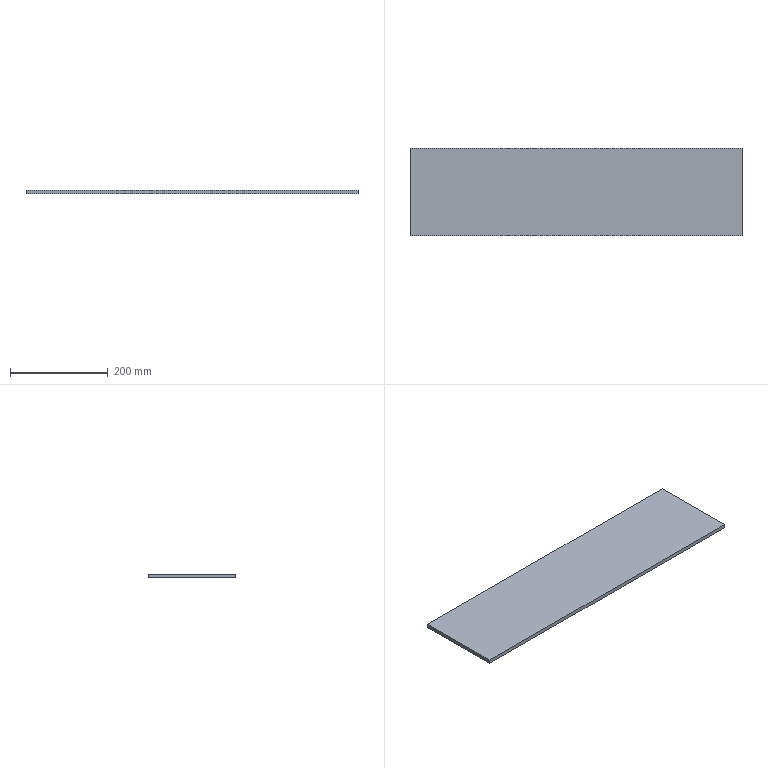Part | STEP file | 04-Steel plate 680x180x8 | 1 solid | 6 faces | box 680 x 180 x 8 mm | volume 979200 mm3 | plane 6
STEP:
#1=CARTESIAN_POINT('',(0.,0.,0.));
#2=DIRECTION('',(0.,0.,1.));
#3=DIRECTION('',(1.,0.,0.));
#4=AXIS2_PLACEMENT_3D('',#1,#2,#3);
#5=CARTESIAN_POINT('',(0.,0.,0.));
#6=VERTEX_POINT('',#5);
#7=CARTESIAN_POINT('',(0.,-180.,0.));
#8=VERTEX_POINT('',#7);
#9=CARTESIAN_POINT('',(0.,0.,0.));
#10=DIRECTION('',(0.,-1.,0.));
#11=VECTOR('',#10,1.);
#12=LINE('',#9,#11);
#13=CARTESIAN_POINT('',(0.,0.,8.));
#14=DIRECTION('',(1.,0.,0.));
#15=DIRECTION('',(0.,1.,0.));
#16=AXIS2_PLACEMENT_3D('',#13,#14,#15);
#17=PLANE('',#16);
#18=CARTESIAN_POINT('',(0.,-8.));
#19=DIRECTION('',(-1.,0.));
#20=VECTOR('',#19,1.);
#21=LINE('',#18,#20);
#22=(GEOMETRIC_REPRESENTATION_CONTEXT(2)PARAMETRIC_REPRESENTATION_CONTEXT()REPRESENTATION_CONTEXT('',''));
#23=DEFINITIONAL_REPRESENTATION('',(#21),#22);
#24=PCURVE('',#17,#23);
#25=CARTESIAN_POINT('',(0.,0.,0.));
#26=DIRECTION('',(0.,0.,1.));
#27=DIRECTION('',(1.,0.,0.));
#28=AXIS2_PLACEMENT_3D('',#25,#26,#27);
#29=PLANE('',#28);
#30=CARTESIAN_POINT('',(0.,0.));
#31=DIRECTION('',(0.,-1.));
#32=VECTOR('',#31,1.);
#33=LINE('',#30,#32);
#34=(GEOMETRIC_REPRESENTATION_CONTEXT(2)PARAMETRIC_REPRESENTATION_CONTEXT()REPRESENTATION_CONTEXT('',''));
#35=DEFINITIONAL_REPRESENTATION('',(#33),#34);
#36=PCURVE('',#29,#35);
#37=SURFACE_CURVE('',#12,(#24,#36),.PCURVE_S1.);
#38=EDGE_CURVE('',#6,#8,#37,.T.);
#39=ORIENTED_EDGE('',*,*,#38,.T.);
#40=CARTESIAN_POINT('',(0.,-180.,8.));
#41=VERTEX_POINT('',#40);
#42=CARTESIAN_POINT('',(0.,-180.,8.));
#43=DIRECTION('',(0.,0.,-1.));
#44=VECTOR('',#43,1.);
#45=LINE('',#42,#44);
#46=CARTESIAN_POINT('',(-180.,0.));
#47=DIRECTION('',(0.,-1.));
#48=VECTOR('',#47,1.);
#49=LINE('',#46,#48);
#50=(GEOMETRIC_REPRESENTATION_CONTEXT(2)PARAMETRIC_REPRESENTATION_CONTEXT()REPRESENTATION_CONTEXT('',''));
#51=DEFINITIONAL_REPRESENTATION('',(#49),#50);
#52=PCURVE('',#17,#51);
#53=CARTESIAN_POINT('',(0.,-180.,8.));
#54=DIRECTION('',(0.,1.,0.));
#55=DIRECTION('',(0.,0.,1.));
#56=AXIS2_PLACEMENT_3D('',#53,#54,#55);
#57=PLANE('',#56);
#58=CARTESIAN_POINT('',(0.,0.));
#59=DIRECTION('',(-1.,0.));
#60=VECTOR('',#59,1.);
#61=LINE('',#58,#60);
#62=(GEOMETRIC_REPRESENTATION_CONTEXT(2)PARAMETRIC_REPRESENTATION_CONTEXT()REPRESENTATION_CONTEXT('',''));
#63=DEFINITIONAL_REPRESENTATION('',(#61),#62);
#64=PCURVE('',#57,#63);
#65=SURFACE_CURVE('',#45,(#52,#64),.PCURVE_S1.);
#66=EDGE_CURVE('',#41,#8,#65,.T.);
#67=ORIENTED_EDGE('',*,*,#66,.F.);
#68=CARTESIAN_POINT('',(0.,0.,8.));
#69=VERTEX_POINT('',#68);
#70=CARTESIAN_POINT('',(0.,0.,8.));
#71=DIRECTION('',(0.,-1.,0.));
#72=VECTOR('',#71,1.);
#73=LINE('',#70,#72);
#74=CARTESIAN_POINT('',(0.,0.));
#75=DIRECTION('',(-1.,0.));
#76=VECTOR('',#75,1.);
#77=LINE('',#74,#76);
#78=(GEOMETRIC_REPRESENTATION_CONTEXT(2)PARAMETRIC_REPRESENTATION_CONTEXT()REPRESENTATION_CONTEXT('',''));
#79=DEFINITIONAL_REPRESENTATION('',(#77),#78);
#80=PCURVE('',#17,#79);
#81=CARTESIAN_POINT('',(0.,0.,8.));
#82=DIRECTION('',(0.,0.,1.));
#83=DIRECTION('',(1.,0.,0.));
#84=AXIS2_PLACEMENT_3D('',#81,#82,#83);
#85=PLANE('',#84);
#86=CARTESIAN_POINT('',(0.,0.));
#87=DIRECTION('',(0.,-1.));
#88=VECTOR('',#87,1.);
#89=LINE('',#86,#88);
#90=(GEOMETRIC_REPRESENTATION_CONTEXT(2)PARAMETRIC_REPRESENTATION_CONTEXT()REPRESENTATION_CONTEXT('',''));
#91=DEFINITIONAL_REPRESENTATION('',(#89),#90);
#92=PCURVE('',#85,#91);
#93=SURFACE_CURVE('',#73,(#80,#92),.PCURVE_S1.);
#94=EDGE_CURVE('',#69,#41,#93,.T.);
#95=ORIENTED_EDGE('',*,*,#94,.F.);
#96=CARTESIAN_POINT('',(0.,0.,8.));
#97=DIRECTION('',(0.,0.,-1.));
#98=VECTOR('',#97,1.);
#99=LINE('',#96,#98);
#100=CARTESIAN_POINT('',(0.,0.));
#101=DIRECTION('',(0.,-1.));
#102=VECTOR('',#101,1.);
#103=LINE('',#100,#102);
#104=(GEOMETRIC_REPRESENTATION_CONTEXT(2)PARAMETRIC_REPRESENTATION_CONTEXT()REPRESENTATION_CONTEXT('',''));
#105=DEFINITIONAL_REPRESENTATION('',(#103),#104);
#106=PCURVE('',#17,#105);
#107=CARTESIAN_POINT('',(0.,0.,8.));
#108=DIRECTION('',(0.,-1.,0.));
#109=DIRECTION('',(0.,0.,-1.));
#110=AXIS2_PLACEMENT_3D('',#107,#108,#109);
#111=PLANE('',#110);
#112=CARTESIAN_POINT('',(0.,0.));
#113=DIRECTION('',(1.,0.));
#114=VECTOR('',#113,1.);
#115=LINE('',#112,#114);
#116=(GEOMETRIC_REPRESENTATION_CONTEXT(2)PARAMETRIC_REPRESENTATION_CONTEXT()REPRESENTATION_CONTEXT('',''));
#117=DEFINITIONAL_REPRESENTATION('',(#115),#116);
#118=PCURVE('',#111,#117);
#119=SURFACE_CURVE('',#99,(#106,#118),.PCURVE_S1.);
#120=EDGE_CURVE('',#69,#6,#119,.T.);
#121=ORIENTED_EDGE('',*,*,#120,.T.);
#122=EDGE_LOOP('',(#39,#67,#95,#121));
#123=FACE_BOUND('',#122,.T.);
#124=ADVANCED_FACE('',(#123),#17,.F.);
#125=CARTESIAN_POINT('',(680.,-180.,0.));
#126=VERTEX_POINT('',#125);
#127=CARTESIAN_POINT('',(0.,-180.,0.));
#128=DIRECTION('',(1.,0.,0.));
#129=VECTOR('',#128,1.);
#130=LINE('',#127,#129);
#131=CARTESIAN_POINT('',(-8.,0.));
#132=DIRECTION('',(0.,1.));
#133=VECTOR('',#132,1.);
#134=LINE('',#131,#133);
#135=(GEOMETRIC_REPRESENTATION_CONTEXT(2)PARAMETRIC_REPRESENTATION_CONTEXT()REPRESENTATION_CONTEXT('',''));
#136=DEFINITIONAL_REPRESENTATION('',(#134),#135);
#137=PCURVE('',#57,#136);
#138=CARTESIAN_POINT('',(0.,-180.));
#139=DIRECTION('',(1.,0.));
#140=VECTOR('',#139,1.);
#141=LINE('',#138,#140);
#142=(GEOMETRIC_REPRESENTATION_CONTEXT(2)PARAMETRIC_REPRESENTATION_CONTEXT()REPRESENTATION_CONTEXT('',''));
#143=DEFINITIONAL_REPRESENTATION('',(#141),#142);
#144=PCURVE('',#29,#143);
#145=SURFACE_CURVE('',#130,(#137,#144),.PCURVE_S1.);
#146=EDGE_CURVE('',#8,#126,#145,.T.);
#147=ORIENTED_EDGE('',*,*,#146,.T.);
#148=CARTESIAN_POINT('',(680.,-180.,8.));
#149=VERTEX_POINT('',#148);
#150=CARTESIAN_POINT('',(680.,-180.,8.));
#151=DIRECTION('',(0.,0.,-1.));
#152=VECTOR('',#151,1.);
#153=LINE('',#150,#152);
#154=CARTESIAN_POINT('',(0.,680.));
#155=DIRECTION('',(-1.,0.));
#156=VECTOR('',#155,1.);
#157=LINE('',#154,#156);
#158=(GEOMETRIC_REPRESENTATION_CONTEXT(2)PARAMETRIC_REPRESENTATION_CONTEXT()REPRESENTATION_CONTEXT('',''));
#159=DEFINITIONAL_REPRESENTATION('',(#157),#158);
#160=PCURVE('',#57,#159);
#161=CARTESIAN_POINT('',(680.,0.,8.));
#162=DIRECTION('',(-1.,0.,0.));
#163=DIRECTION('',(0.,0.,1.));
#164=AXIS2_PLACEMENT_3D('',#161,#162,#163);
#165=PLANE('',#164);
#166=CARTESIAN_POINT('',(0.,-180.));
#167=DIRECTION('',(-1.,0.));
#168=VECTOR('',#167,1.);
#169=LINE('',#166,#168);
#170=(GEOMETRIC_REPRESENTATION_CONTEXT(2)PARAMETRIC_REPRESENTATION_CONTEXT()REPRESENTATION_CONTEXT('',''));
#171=DEFINITIONAL_REPRESENTATION('',(#169),#170);
#172=PCURVE('',#165,#171);
#173=SURFACE_CURVE('',#153,(#160,#172),.PCURVE_S1.);
#174=EDGE_CURVE('',#149,#126,#173,.T.);
#175=ORIENTED_EDGE('',*,*,#174,.F.);
#176=CARTESIAN_POINT('',(0.,-180.,8.));
#177=DIRECTION('',(1.,0.,0.));
#178=VECTOR('',#177,1.);
#179=LINE('',#176,#178);
#180=CARTESIAN_POINT('',(0.,0.));
#181=DIRECTION('',(0.,1.));
#182=VECTOR('',#181,1.);
#183=LINE('',#180,#182);
#184=(GEOMETRIC_REPRESENTATION_CONTEXT(2)PARAMETRIC_REPRESENTATION_CONTEXT()REPRESENTATION_CONTEXT('',''));
#185=DEFINITIONAL_REPRESENTATION('',(#183),#184);
#186=PCURVE('',#57,#185);
#187=CARTESIAN_POINT('',(0.,-180.));
#188=DIRECTION('',(1.,0.));
#189=VECTOR('',#188,1.);
#190=LINE('',#187,#189);
#191=(GEOMETRIC_REPRESENTATION_CONTEXT(2)PARAMETRIC_REPRESENTATION_CONTEXT()REPRESENTATION_CONTEXT('',''));
#192=DEFINITIONAL_REPRESENTATION('',(#190),#191);
#193=PCURVE('',#85,#192);
#194=SURFACE_CURVE('',#179,(#186,#193),.PCURVE_S1.);
#195=EDGE_CURVE('',#41,#149,#194,.T.);
#196=ORIENTED_EDGE('',*,*,#195,.F.);
#197=ORIENTED_EDGE('',*,*,#66,.T.);
#198=EDGE_LOOP('',(#147,#175,#196,#197));
#199=FACE_BOUND('',#198,.T.);
#200=ADVANCED_FACE('',(#199),#57,.F.);
#201=CARTESIAN_POINT('',(680.,0.,0.));
#202=VERTEX_POINT('',#201);
#203=CARTESIAN_POINT('',(680.,0.,0.));
#204=DIRECTION('',(0.,1.,0.));
#205=VECTOR('',#204,1.);
#206=LINE('',#203,#205);
#207=CARTESIAN_POINT('',(-8.,0.));
#208=DIRECTION('',(0.,1.));
#209=VECTOR('',#208,1.);
#210=LINE('',#207,#209);
#211=(GEOMETRIC_REPRESENTATION_CONTEXT(2)PARAMETRIC_REPRESENTATION_CONTEXT()REPRESENTATION_CONTEXT('',''));
#212=DEFINITIONAL_REPRESENTATION('',(#210),#211);
#213=PCURVE('',#165,#212);
#214=CARTESIAN_POINT('',(680.,0.));
#215=DIRECTION('',(0.,1.));
#216=VECTOR('',#215,1.);
#217=LINE('',#214,#216);
#218=(GEOMETRIC_REPRESENTATION_CONTEXT(2)PARAMETRIC_REPRESENTATION_CONTEXT()REPRESENTATION_CONTEXT('',''));
#219=DEFINITIONAL_REPRESENTATION('',(#217),#218);
#220=PCURVE('',#29,#219);
#221=SURFACE_CURVE('',#206,(#213,#220),.PCURVE_S1.);
#222=EDGE_CURVE('',#126,#202,#221,.T.);
#223=ORIENTED_EDGE('',*,*,#222,.T.);
#224=CARTESIAN_POINT('',(680.,0.,8.));
#225=VERTEX_POINT('',#224);
#226=CARTESIAN_POINT('',(680.,0.,8.));
#227=DIRECTION('',(0.,0.,-1.));
#228=VECTOR('',#227,1.);
#229=LINE('',#226,#228);
#230=CARTESIAN_POINT('',(0.,0.));
#231=DIRECTION('',(-1.,0.));
#232=VECTOR('',#231,1.);
#233=LINE('',#230,#232);
#234=(GEOMETRIC_REPRESENTATION_CONTEXT(2)PARAMETRIC_REPRESENTATION_CONTEXT()REPRESENTATION_CONTEXT('',''));
#235=DEFINITIONAL_REPRESENTATION('',(#233),#234);
#236=PCURVE('',#165,#235);
#237=CARTESIAN_POINT('',(0.,680.));
#238=DIRECTION('',(1.,0.));
#239=VECTOR('',#238,1.);
#240=LINE('',#237,#239);
#241=(GEOMETRIC_REPRESENTATION_CONTEXT(2)PARAMETRIC_REPRESENTATION_CONTEXT()REPRESENTATION_CONTEXT('',''));
#242=DEFINITIONAL_REPRESENTATION('',(#240),#241);
#243=PCURVE('',#111,#242);
#244=SURFACE_CURVE('',#229,(#236,#243),.PCURVE_S1.);
#245=EDGE_CURVE('',#225,#202,#244,.T.);
#246=ORIENTED_EDGE('',*,*,#245,.F.);
#247=CARTESIAN_POINT('',(680.,0.,8.));
#248=DIRECTION('',(0.,1.,0.));
#249=VECTOR('',#248,1.);
#250=LINE('',#247,#249);
#251=CARTESIAN_POINT('',(0.,0.));
#252=DIRECTION('',(0.,1.));
#253=VECTOR('',#252,1.);
#254=LINE('',#251,#253);
#255=(GEOMETRIC_REPRESENTATION_CONTEXT(2)PARAMETRIC_REPRESENTATION_CONTEXT()REPRESENTATION_CONTEXT('',''));
#256=DEFINITIONAL_REPRESENTATION('',(#254),#255);
#257=PCURVE('',#165,#256);
#258=CARTESIAN_POINT('',(680.,0.));
#259=DIRECTION('',(0.,1.));
#260=VECTOR('',#259,1.);
#261=LINE('',#258,#260);
#262=(GEOMETRIC_REPRESENTATION_CONTEXT(2)PARAMETRIC_REPRESENTATION_CONTEXT()REPRESENTATION_CONTEXT('',''));
#263=DEFINITIONAL_REPRESENTATION('',(#261),#262);
#264=PCURVE('',#85,#263);
#265=SURFACE_CURVE('',#250,(#257,#264),.PCURVE_S1.);
#266=EDGE_CURVE('',#149,#225,#265,.T.);
#267=ORIENTED_EDGE('',*,*,#266,.F.);
#268=ORIENTED_EDGE('',*,*,#174,.T.);
#269=EDGE_LOOP('',(#223,#246,#267,#268));
#270=FACE_BOUND('',#269,.T.);
#271=ADVANCED_FACE('',(#270),#165,.F.);
#272=CARTESIAN_POINT('',(0.,0.,0.));
#273=DIRECTION('',(-1.,0.,0.));
#274=VECTOR('',#273,1.);
#275=LINE('',#272,#274);
#276=CARTESIAN_POINT('',(8.,0.));
#277=DIRECTION('',(0.,-1.));
#278=VECTOR('',#277,1.);
#279=LINE('',#276,#278);
#280=(GEOMETRIC_REPRESENTATION_CONTEXT(2)PARAMETRIC_REPRESENTATION_CONTEXT()REPRESENTATION_CONTEXT('',''));
#281=DEFINITIONAL_REPRESENTATION('',(#279),#280);
#282=PCURVE('',#111,#281);
#283=CARTESIAN_POINT('',(0.,0.));
#284=DIRECTION('',(-1.,0.));
#285=VECTOR('',#284,1.);
#286=LINE('',#283,#285);
#287=(GEOMETRIC_REPRESENTATION_CONTEXT(2)PARAMETRIC_REPRESENTATION_CONTEXT()REPRESENTATION_CONTEXT('',''));
#288=DEFINITIONAL_REPRESENTATION('',(#286),#287);
#289=PCURVE('',#29,#288);
#290=SURFACE_CURVE('',#275,(#282,#289),.PCURVE_S1.);
#291=EDGE_CURVE('',#202,#6,#290,.T.);
#292=ORIENTED_EDGE('',*,*,#291,.T.);
#293=ORIENTED_EDGE('',*,*,#120,.F.);
#294=CARTESIAN_POINT('',(0.,0.,8.));
#295=DIRECTION('',(-1.,0.,0.));
#296=VECTOR('',#295,1.);
#297=LINE('',#294,#296);
#298=CARTESIAN_POINT('',(0.,0.));
#299=DIRECTION('',(0.,-1.));
#300=VECTOR('',#299,1.);
#301=LINE('',#298,#300);
#302=(GEOMETRIC_REPRESENTATION_CONTEXT(2)PARAMETRIC_REPRESENTATION_CONTEXT()REPRESENTATION_CONTEXT('',''));
#303=DEFINITIONAL_REPRESENTATION('',(#301),#302);
#304=PCURVE('',#111,#303);
#305=CARTESIAN_POINT('',(0.,0.));
#306=DIRECTION('',(-1.,0.));
#307=VECTOR('',#306,1.);
#308=LINE('',#305,#307);
#309=(GEOMETRIC_REPRESENTATION_CONTEXT(2)PARAMETRIC_REPRESENTATION_CONTEXT()REPRESENTATION_CONTEXT('',''));
#310=DEFINITIONAL_REPRESENTATION('',(#308),#309);
#311=PCURVE('',#85,#310);
#312=SURFACE_CURVE('',#297,(#304,#311),.PCURVE_S1.);
#313=EDGE_CURVE('',#225,#69,#312,.T.);
#314=ORIENTED_EDGE('',*,*,#313,.F.);
#315=ORIENTED_EDGE('',*,*,#245,.T.);
#316=EDGE_LOOP('',(#292,#293,#314,#315));
#317=FACE_BOUND('',#316,.T.);
#318=ADVANCED_FACE('',(#317),#111,.F.);
#319=ORIENTED_EDGE('',*,*,#94,.T.);
#320=ORIENTED_EDGE('',*,*,#195,.T.);
#321=ORIENTED_EDGE('',*,*,#266,.T.);
#322=ORIENTED_EDGE('',*,*,#313,.T.);
#323=EDGE_LOOP('',(#319,#320,#321,#322));
#324=FACE_BOUND('',#323,.T.);
#325=ADVANCED_FACE('',(#324),#85,.T.);
#326=ORIENTED_EDGE('',*,*,#38,.F.);
#327=ORIENTED_EDGE('',*,*,#291,.F.);
#328=ORIENTED_EDGE('',*,*,#222,.F.);
#329=ORIENTED_EDGE('',*,*,#146,.F.);
#330=EDGE_LOOP('',(#326,#327,#328,#329));
#331=FACE_BOUND('',#330,.T.);
#332=ADVANCED_FACE('',(#331),#29,.F.);
#333=CLOSED_SHELL('',(#124,#200,#271,#318,#325,#332));
#334=MANIFOLD_SOLID_BREP('',#333);
#335=(LENGTH_UNIT()NAMED_UNIT(*)SI_UNIT(.MILLI.,.METRE.));
#336=UNCERTAINTY_MEASURE_WITH_UNIT(LENGTH_MEASURE(0.0000001),#335,'','');
#337=(NAMED_UNIT(*)PLANE_ANGLE_UNIT()SI_UNIT($,.RADIAN.));
#338=(NAMED_UNIT(*)SI_UNIT($,.STERADIAN.)SOLID_ANGLE_UNIT());
#339=(GEOMETRIC_REPRESENTATION_CONTEXT(3)GLOBAL_UNCERTAINTY_ASSIGNED_CONTEXT((#336))GLOBAL_UNIT_ASSIGNED_CONTEXT((#335,#337,#338))REPRESENTATION_CONTEXT('',''));
#340=ADVANCED_BREP_SHAPE_REPRESENTATION('',(#4,#334),#339);